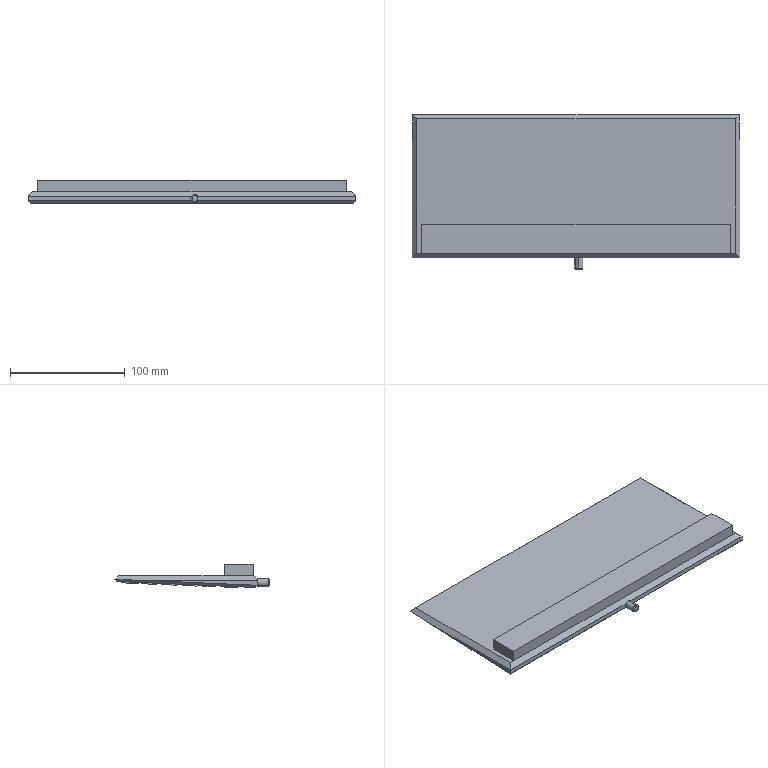Part | STEP file | computer numeric keypad HW098A | 1 solid | 427 faces | box 285 x 134.477 x 20.707 mm | volume 348145 mm3 | plane 423 | torus 2 | cylinder 2 | commonest cylinder face diameters 7 x2